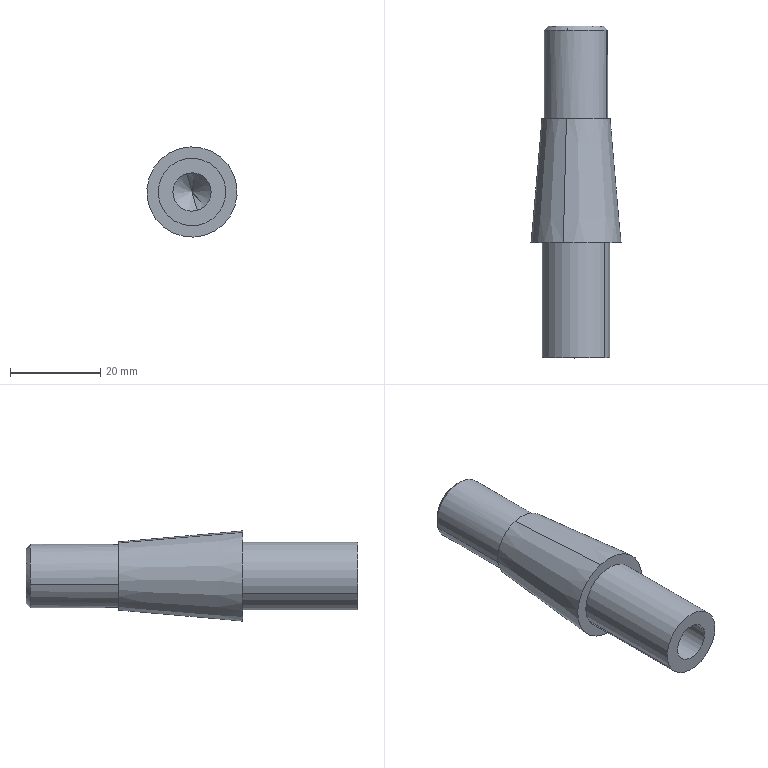Part | SolidWorks | features BaseBody 1 | 1 solid | 16 faces | box 20 x 73.5 x 20 mm | volume 13373 mm3 | cone 6 | cylinder 6 | plane 4 | commonest cylinder face diameters 8.5 x2 14 x2 14.95 x2
STEP:
#1=CARTESIAN_POINT('',(-385.826,-48.,37.663));
#2=VERTEX_POINT('',#1);
#3=CARTESIAN_POINT('',(-389.222,-48.,49.277));
#4=VERTEX_POINT('',#3);
#5=CARTESIAN_POINT('',(-387.524,-48.,43.47));
#6=DIRECTION('',(0.,1.,0.));
#7=DIRECTION('',(-0.9598,0.,-0.2807));
#8=AXIS2_PLACEMENT_3D('',#5,#6,#7);
#9=CIRCLE('',#8,6.05);
#10=EDGE_CURVE('',#2,#4,#9,.T.);
#11=ORIENTED_EDGE('',*,*,#10,.F.);
#12=CARTESIAN_POINT('',(-385.56,-48.95,36.751));
#13=VERTEX_POINT('',#12);
#14=CARTESIAN_POINT('',(-385.693,-48.475,37.207));
#15=DIRECTION('',(0.1985,-0.7071,-0.6787));
#16=VECTOR('',#15,1000.);
#17=LINE('',#14,#16);
#18=EDGE_CURVE('',#2,#13,#17,.T.);
#19=ORIENTED_EDGE('',*,*,#18,.T.);
#20=CARTESIAN_POINT('',(-394.243,-48.95,41.505));
#21=VERTEX_POINT('',#20);
#22=CARTESIAN_POINT('',(-387.524,-48.95,43.47));
#23=DIRECTION('',(0.,1.,0.));
#24=DIRECTION('',(-0.9598,0.,-0.2807));
#25=AXIS2_PLACEMENT_3D('',#22,#23,#24);
#26=CIRCLE('',#25,7.);
#27=EDGE_CURVE('',#13,#21,#26,.T.);
#28=ORIENTED_EDGE('',*,*,#27,.T.);
#29=CARTESIAN_POINT('',(-389.489,-48.95,50.189));
#30=VERTEX_POINT('',#29);
#31=CARTESIAN_POINT('',(-387.524,-48.95,43.47));
#32=DIRECTION('',(0.,1.,0.));
#33=DIRECTION('',(-0.9598,0.,-0.2807));
#34=AXIS2_PLACEMENT_3D('',#31,#32,#33);
#35=CIRCLE('',#34,7.);
#36=EDGE_CURVE('',#21,#30,#35,.T.);
#37=ORIENTED_EDGE('',*,*,#36,.T.);
#38=CARTESIAN_POINT('',(-389.356,-48.475,49.733));
#39=DIRECTION('',(-0.1985,-0.7071,0.6787));
#40=VECTOR('',#39,1000.);
#41=LINE('',#38,#40);
#42=EDGE_CURVE('',#4,#30,#41,.T.);
#43=ORIENTED_EDGE('',*,*,#42,.F.);
#44=EDGE_LOOP('',(#11,#19,#28,#37,#43));
#45=FACE_OUTER_BOUND('',#44,.T.);
#46=CARTESIAN_POINT('',(-387.524,-48.475,43.47));
#47=DIRECTION('',(0.,-1.,0.));
#48=DIRECTION('',(-0.2807,0.,0.9598));
#49=AXIS2_PLACEMENT_3D('',#46,#47,#48);
#50=CONICAL_SURFACE('',#49,6.525,0.7854);
#51=ADVANCED_FACE('',(#45),#50,.T.);
#52=CARTESIAN_POINT('',(-387.524,-102.,43.47));
#53=VERTEX_POINT('',#52);
#54=CARTESIAN_POINT('',(-388.717,-106.25,47.549));
#55=VERTEX_POINT('',#54);
#56=CARTESIAN_POINT('',(-388.133,-104.168,45.55));
#57=DIRECTION('',(-0.1985,-0.7071,0.6787));
#58=VECTOR('',#57,1000.);
#59=LINE('',#56,#58);
#60=EDGE_CURVE('',#53,#55,#59,.T.);
#61=ORIENTED_EDGE('',*,*,#60,.F.);
#62=CARTESIAN_POINT('',(-386.332,-106.25,39.391));
#63=VERTEX_POINT('',#62);
#64=CARTESIAN_POINT('',(-386.916,-104.168,41.39));
#65=DIRECTION('',(0.1985,-0.7071,-0.6787));
#66=VECTOR('',#65,1000.);
#67=LINE('',#64,#66);
#68=EDGE_CURVE('',#53,#63,#67,.T.);
#69=ORIENTED_EDGE('',*,*,#68,.T.);
#70=CARTESIAN_POINT('',(-383.445,-106.25,44.663));
#71=VERTEX_POINT('',#70);
#72=CARTESIAN_POINT('',(-387.524,-106.25,43.47));
#73=DIRECTION('',(0.,1.,0.));
#74=DIRECTION('',(-0.9598,0.,-0.2807));
#75=AXIS2_PLACEMENT_3D('',#72,#73,#74);
#76=CIRCLE('',#75,4.25);
#77=EDGE_CURVE('',#71,#63,#76,.T.);
#78=ORIENTED_EDGE('',*,*,#77,.F.);
#79=CARTESIAN_POINT('',(-387.524,-106.25,43.47));
#80=DIRECTION('',(0.,1.,0.));
#81=DIRECTION('',(-0.9598,0.,-0.2807));
#82=AXIS2_PLACEMENT_3D('',#79,#80,#81);
#83=CIRCLE('',#82,4.25);
#84=EDGE_CURVE('',#55,#71,#83,.T.);
#85=ORIENTED_EDGE('',*,*,#84,.F.);
#86=EDGE_LOOP('',(#61,#69,#78,#85));
#87=FACE_OUTER_BOUND('',#86,.T.);
#88=CARTESIAN_POINT('',(-387.524,-104.168,43.47));
#89=DIRECTION('',(0.,-1.,0.));
#90=DIRECTION('',(-0.2807,0.,0.9598));
#91=AXIS2_PLACEMENT_3D('',#88,#89,#90);
#92=CONICAL_SURFACE('',#91,2.168,0.7854);
#93=ADVANCED_FACE('',(#87),#92,.F.);
#94=CARTESIAN_POINT('',(-391.604,-106.25,42.277));
#95=VERTEX_POINT('',#94);
#96=CARTESIAN_POINT('',(-387.524,-106.25,43.47));
#97=DIRECTION('',(0.,1.,0.));
#98=DIRECTION('',(-0.9598,0.,-0.2807));
#99=AXIS2_PLACEMENT_3D('',#96,#97,#98);
#100=CIRCLE('',#99,4.25);
#101=EDGE_CURVE('',#95,#55,#100,.T.);
#102=ORIENTED_EDGE('',*,*,#101,.T.);
#103=ORIENTED_EDGE('',*,*,#84,.T.);
#104=CARTESIAN_POINT('',(-383.445,-121.5,44.663));
#105=VERTEX_POINT('',#104);
#106=CARTESIAN_POINT('',(-383.445,-122.,44.663));
#107=DIRECTION('',(0.,-1.,0.));
#108=VECTOR('',#107,1000.);
#109=LINE('',#106,#108);
#110=EDGE_CURVE('',#71,#105,#109,.T.);
#111=ORIENTED_EDGE('',*,*,#110,.T.);
#112=CARTESIAN_POINT('',(-391.604,-121.5,42.277));
#113=VERTEX_POINT('',#112);
#114=CARTESIAN_POINT('',(-387.524,-121.5,43.47));
#115=DIRECTION('',(0.,1.,0.));
#116=DIRECTION('',(-0.9598,0.,-0.2807));
#117=AXIS2_PLACEMENT_3D('',#114,#115,#116);
#118=CIRCLE('',#117,4.25);
#119=EDGE_CURVE('',#113,#105,#118,.T.);
#120=ORIENTED_EDGE('',*,*,#119,.F.);
#121=CARTESIAN_POINT('',(-391.604,-122.,42.277));
#122=DIRECTION('',(0.,-1.,0.));
#123=VECTOR('',#122,1000.);
#124=LINE('',#121,#123);
#125=EDGE_CURVE('',#95,#113,#124,.T.);
#126=ORIENTED_EDGE('',*,*,#125,.F.);
#127=EDGE_LOOP('',(#102,#103,#111,#120,#126));
#128=FACE_OUTER_BOUND('',#127,.T.);
#129=CARTESIAN_POINT('',(-387.524,-122.,43.47));
#130=DIRECTION('',(0.,-1.,0.));
#131=DIRECTION('',(-0.9598,0.,-0.2807));
#132=AXIS2_PLACEMENT_3D('',#129,#130,#131);
#133=CYLINDRICAL_SURFACE('',#132,4.25);
#134=ADVANCED_FACE('',(#128),#133,.F.);
#135=CARTESIAN_POINT('',(-381.159,-96.,47.389));
#136=VERTEX_POINT('',#135);
#137=CARTESIAN_POINT('',(-393.89,-96.,39.551));
#138=VERTEX_POINT('',#137);
#139=CARTESIAN_POINT('',(-387.524,-96.,43.47));
#140=DIRECTION('',(0.,1.,0.));
#141=DIRECTION('',(0.8515,0.,0.5243));
#142=AXIS2_PLACEMENT_3D('',#139,#140,#141);
#143=CIRCLE('',#142,7.475);
#144=EDGE_CURVE('',#136,#138,#143,.T.);
#145=ORIENTED_EDGE('',*,*,#144,.F.);
#146=CARTESIAN_POINT('',(-381.159,-121.5,47.389));
#147=VERTEX_POINT('',#146);
#148=CARTESIAN_POINT('',(-381.159,-122.,47.389));
#149=DIRECTION('',(0.,-1.,0.));
#150=VECTOR('',#149,1000.);
#151=LINE('',#148,#150);
#152=EDGE_CURVE('',#136,#147,#151,.T.);
#153=ORIENTED_EDGE('',*,*,#152,.T.);
#154=CARTESIAN_POINT('',(-393.89,-121.5,39.551));
#155=VERTEX_POINT('',#154);
#156=CARTESIAN_POINT('',(-387.524,-121.5,43.47));
#157=DIRECTION('',(0.,-1.,0.));
#158=DIRECTION('',(0.,0.,-1.));
#159=AXIS2_PLACEMENT_3D('',#156,#157,#158);
#160=CIRCLE('',#159,7.475);
#161=EDGE_CURVE('',#155,#147,#160,.T.);
#162=ORIENTED_EDGE('',*,*,#161,.F.);
#163=CARTESIAN_POINT('',(-393.89,-122.,39.551));
#164=DIRECTION('',(0.,-1.,0.));
#165=VECTOR('',#164,1000.);
#166=LINE('',#163,#165);
#167=EDGE_CURVE('',#138,#155,#166,.T.);
#168=ORIENTED_EDGE('',*,*,#167,.F.);
#169=EDGE_LOOP('',(#145,#153,#162,#168));
#170=FACE_OUTER_BOUND('',#169,.T.);
#171=CARTESIAN_POINT('',(-387.524,-122.,43.47));
#172=DIRECTION('',(0.,-1.,0.));
#173=DIRECTION('',(-0.8515,0.,-0.5243));
#174=AXIS2_PLACEMENT_3D('',#171,#172,#173);
#175=CYLINDRICAL_SURFACE('',#174,7.475);
#176=ADVANCED_FACE('',(#170),#175,.T.);
#177=CARTESIAN_POINT('',(-394.243,-68.5,41.505));
#178=VERTEX_POINT('',#177);
#179=CARTESIAN_POINT('',(-380.806,-68.5,45.435));
#180=VERTEX_POINT('',#179);
#181=CARTESIAN_POINT('',(-387.524,-68.5,43.47));
#182=DIRECTION('',(0.,-1.,0.));
#183=DIRECTION('',(0.9598,0.,0.2807));
#184=AXIS2_PLACEMENT_3D('',#181,#182,#183);
#185=CIRCLE('',#184,7.);
#186=EDGE_CURVE('',#178,#180,#185,.T.);
#187=ORIENTED_EDGE('',*,*,#186,.F.);
#188=CARTESIAN_POINT('',(-394.243,-63.,41.505));
#189=DIRECTION('',(0.,1.,0.));
#190=VECTOR('',#189,1000.);
#191=LINE('',#188,#190);
#192=EDGE_CURVE('',#178,#21,#191,.T.);
#193=ORIENTED_EDGE('',*,*,#192,.T.);
#194=ORIENTED_EDGE('',*,*,#27,.F.);
#195=CARTESIAN_POINT('',(-380.806,-48.95,45.435));
#196=VERTEX_POINT('',#195);
#197=CARTESIAN_POINT('',(-387.524,-48.95,43.47));
#198=DIRECTION('',(0.,1.,0.));
#199=DIRECTION('',(-0.9598,0.,-0.2807));
#200=AXIS2_PLACEMENT_3D('',#197,#198,#199);
#201=CIRCLE('',#200,7.);
#202=EDGE_CURVE('',#196,#13,#201,.T.);
#203=ORIENTED_EDGE('',*,*,#202,.F.);
#204=CARTESIAN_POINT('',(-380.806,-63.,45.435));
#205=DIRECTION('',(0.,1.,0.));
#206=VECTOR('',#205,1000.);
#207=LINE('',#204,#206);
#208=EDGE_CURVE('',#180,#196,#207,.T.);
#209=ORIENTED_EDGE('',*,*,#208,.F.);
#210=EDGE_LOOP('',(#187,#193,#194,#203,#209));
#211=FACE_OUTER_BOUND('',#210,.T.);
#212=CARTESIAN_POINT('',(-387.524,-63.,43.47));
#213=DIRECTION('',(0.,1.,0.));
#214=DIRECTION('',(0.9598,0.,0.2807));
#215=AXIS2_PLACEMENT_3D('',#212,#213,#214);
#216=CYLINDRICAL_SURFACE('',#215,7.);
#217=ADVANCED_FACE('',(#211),#216,.T.);
#218=CARTESIAN_POINT('',(-389.647,-68.5,50.73));
#219=VERTEX_POINT('',#218);
#220=CARTESIAN_POINT('',(-385.402,-68.5,36.21));
#221=VERTEX_POINT('',#220);
#222=CARTESIAN_POINT('',(-387.524,-68.5,43.47));
#223=DIRECTION('',(0.,-1.,0.));
#224=DIRECTION('',(-0.2807,0.,0.9598));
#225=AXIS2_PLACEMENT_3D('',#222,#223,#224);
#226=CIRCLE('',#225,7.564);
#227=EDGE_CURVE('',#219,#221,#226,.T.);
#228=ORIENTED_EDGE('',*,*,#227,.T.);
#229=CARTESIAN_POINT('',(-384.718,-96.,33.872));
#230=VERTEX_POINT('',#229);
#231=CARTESIAN_POINT('',(-385.06,-82.25,35.041));
#232=DIRECTION('',(0.02477,-0.9961,-0.0847));
#233=VECTOR('',#232,1000.);
#234=LINE('',#231,#233);
#235=EDGE_CURVE('',#221,#230,#234,.T.);
#236=ORIENTED_EDGE('',*,*,#235,.T.);
#237=CARTESIAN_POINT('',(-390.331,-96.,53.068));
#238=VERTEX_POINT('',#237);
#239=CARTESIAN_POINT('',(-387.524,-96.,43.47));
#240=DIRECTION('',(0.,-1.,0.));
#241=DIRECTION('',(0.2807,0.,-0.9598));
#242=AXIS2_PLACEMENT_3D('',#239,#240,#241);
#243=CIRCLE('',#242,10.);
#244=EDGE_CURVE('',#238,#230,#243,.T.);
#245=ORIENTED_EDGE('',*,*,#244,.F.);
#246=CARTESIAN_POINT('',(-389.989,-82.25,51.899));
#247=DIRECTION('',(-0.02477,-0.9961,0.0847));
#248=VECTOR('',#247,1000.);
#249=LINE('',#246,#248);
#250=EDGE_CURVE('',#219,#238,#249,.T.);
#251=ORIENTED_EDGE('',*,*,#250,.F.);
#252=EDGE_LOOP('',(#228,#236,#245,#251));
#253=FACE_OUTER_BOUND('',#252,.T.);
#254=CARTESIAN_POINT('',(-387.524,-82.25,43.47));
#255=DIRECTION('',(0.,-1.,0.));
#256=DIRECTION('',(-0.2807,0.,0.9598));
#257=AXIS2_PLACEMENT_3D('',#254,#255,#256);
#258=CONICAL_SURFACE('',#257,8.782,0.08837);
#259=ADVANCED_FACE('',(#253),#258,.T.);
#260=ORIENTED_EDGE('',*,*,#119,.T.);
#261=CARTESIAN_POINT('',(-387.524,-121.5,43.47));
#262=DIRECTION('',(0.,1.,0.));
#263=DIRECTION('',(-0.9598,0.,-0.2807));
#264=AXIS2_PLACEMENT_3D('',#261,#262,#263);
#265=CIRCLE('',#264,4.25);
#266=EDGE_CURVE('',#105,#113,#265,.T.);
#267=ORIENTED_EDGE('',*,*,#266,.T.);
#268=EDGE_LOOP('',(#260,#267));
#269=FACE_BOUND('',#268,.T.);
#270=ORIENTED_EDGE('',*,*,#161,.T.);
#271=CARTESIAN_POINT('',(-387.524,-121.5,43.47));
#272=DIRECTION('',(0.,-1.,0.));
#273=DIRECTION('',(0.,0.,-1.));
#274=AXIS2_PLACEMENT_3D('',#271,#272,#273);
#275=CIRCLE('',#274,7.475);
#276=EDGE_CURVE('',#147,#155,#275,.T.);
#277=ORIENTED_EDGE('',*,*,#276,.T.);
#278=EDGE_LOOP('',(#270,#277));
#279=FACE_OUTER_BOUND('',#278,.T.);
#280=CARTESIAN_POINT('',(-449.261,-121.5,5.459));
#281=DIRECTION('',(0.,-1.,0.));
#282=DIRECTION('',(0.,0.,-1.));
#283=AXIS2_PLACEMENT_3D('',#280,#281,#282);
#284=PLANE('',#283);
#285=ADVANCED_FACE('',(#269,#279),#284,.T.);
#286=CARTESIAN_POINT('',(-387.524,-96.,43.47));
#287=DIRECTION('',(0.,1.,0.));
#288=DIRECTION('',(0.8515,0.,0.5243));
#289=AXIS2_PLACEMENT_3D('',#286,#287,#288);
#290=CIRCLE('',#289,7.475);
#291=EDGE_CURVE('',#138,#136,#290,.T.);
#292=ORIENTED_EDGE('',*,*,#291,.T.);
#293=ORIENTED_EDGE('',*,*,#144,.T.);
#294=EDGE_LOOP('',(#292,#293));
#295=FACE_BOUND('',#294,.T.);
#296=ORIENTED_EDGE('',*,*,#244,.T.);
#297=CARTESIAN_POINT('',(-387.524,-96.,43.47));
#298=DIRECTION('',(0.,-1.,0.));
#299=DIRECTION('',(0.2807,0.,-0.9598));
#300=AXIS2_PLACEMENT_3D('',#297,#298,#299);
#301=CIRCLE('',#300,10.);
#302=EDGE_CURVE('',#230,#238,#301,.T.);
#303=ORIENTED_EDGE('',*,*,#302,.T.);
#304=EDGE_LOOP('',(#296,#303));
#305=FACE_OUTER_BOUND('',#304,.T.);
#306=CARTESIAN_POINT('',(-387.524,-96.,43.47));
#307=DIRECTION('',(0.,-1.,0.));
#308=DIRECTION('',(0.,0.,-1.));
#309=AXIS2_PLACEMENT_3D('',#306,#307,#308);
#310=PLANE('',#309);
#311=ADVANCED_FACE('',(#295,#305),#310,.T.);
#312=ORIENTED_EDGE('',*,*,#235,.F.);
#313=CARTESIAN_POINT('',(-387.524,-68.5,43.47));
#314=DIRECTION('',(0.,-1.,0.));
#315=DIRECTION('',(-0.2807,0.,0.9598));
#316=AXIS2_PLACEMENT_3D('',#313,#314,#315);
#317=CIRCLE('',#316,7.564);
#318=EDGE_CURVE('',#221,#219,#317,.T.);
#319=ORIENTED_EDGE('',*,*,#318,.T.);
#320=ORIENTED_EDGE('',*,*,#250,.T.);
#321=ORIENTED_EDGE('',*,*,#302,.F.);
#322=EDGE_LOOP('',(#312,#319,#320,#321));
#323=FACE_OUTER_BOUND('',#322,.T.);
#324=CARTESIAN_POINT('',(-387.524,-82.25,43.47));
#325=DIRECTION('',(0.,-1.,0.));
#326=DIRECTION('',(-0.2807,0.,0.9598));
#327=AXIS2_PLACEMENT_3D('',#324,#325,#326);
#328=CONICAL_SURFACE('',#327,8.782,0.08837);
#329=ADVANCED_FACE('',(#323),#328,.T.);
#330=CARTESIAN_POINT('',(-387.524,-68.5,43.47));
#331=DIRECTION('',(0.,-1.,0.));
#332=DIRECTION('',(0.9598,0.,0.2807));
#333=AXIS2_PLACEMENT_3D('',#330,#331,#332);
#334=CIRCLE('',#333,7.);
#335=EDGE_CURVE('',#180,#178,#334,.T.);
#336=ORIENTED_EDGE('',*,*,#335,.T.);
#337=ORIENTED_EDGE('',*,*,#186,.T.);
#338=EDGE_LOOP('',(#336,#337));
#339=FACE_BOUND('',#338,.T.);
#340=ORIENTED_EDGE('',*,*,#227,.F.);
#341=ORIENTED_EDGE('',*,*,#318,.F.);
#342=EDGE_LOOP('',(#340,#341));
#343=FACE_OUTER_BOUND('',#342,.T.);
#344=CARTESIAN_POINT('',(5.879,-68.5,101.935));
#345=DIRECTION('',(0.,1.,0.));
#346=DIRECTION('',(1.,0.,0.));
#347=AXIS2_PLACEMENT_3D('',#344,#345,#346);
#348=PLANE('',#347);
#349=ADVANCED_FACE('',(#339,#343),#348,.T.);
#350=ORIENTED_EDGE('',*,*,#192,.F.);
#351=ORIENTED_EDGE('',*,*,#335,.F.);
#352=ORIENTED_EDGE('',*,*,#208,.T.);
#353=CARTESIAN_POINT('',(-387.524,-48.95,43.47));
#354=DIRECTION('',(0.,1.,0.));
#355=DIRECTION('',(-0.9598,0.,-0.2807));
#356=AXIS2_PLACEMENT_3D('',#353,#354,#355);
#357=CIRCLE('',#356,7.);
#358=EDGE_CURVE('',#30,#196,#357,.T.);
#359=ORIENTED_EDGE('',*,*,#358,.F.);
#360=ORIENTED_EDGE('',*,*,#36,.F.);
#361=EDGE_LOOP('',(#350,#351,#352,#359,#360));
#362=FACE_OUTER_BOUND('',#361,.T.);
#363=CARTESIAN_POINT('',(-387.524,-63.,43.47));
#364=DIRECTION('',(0.,1.,0.));
#365=DIRECTION('',(0.9598,0.,0.2807));
#366=AXIS2_PLACEMENT_3D('',#363,#364,#365);
#367=CYLINDRICAL_SURFACE('',#366,7.);
#368=ADVANCED_FACE('',(#362),#367,.T.);
#369=CARTESIAN_POINT('',(-387.524,-48.,43.47));
#370=DIRECTION('',(0.,1.,0.));
#371=DIRECTION('',(-0.9598,0.,-0.2807));
#372=AXIS2_PLACEMENT_3D('',#369,#370,#371);
#373=CIRCLE('',#372,6.05);
#374=EDGE_CURVE('',#4,#2,#373,.T.);
#375=ORIENTED_EDGE('',*,*,#374,.T.);
#376=ORIENTED_EDGE('',*,*,#10,.T.);
#377=EDGE_LOOP('',(#375,#376));
#378=FACE_OUTER_BOUND('',#377,.T.);
#379=CARTESIAN_POINT('',(5.879,-48.,101.935));
#380=DIRECTION('',(0.,1.,0.));
#381=DIRECTION('',(1.,0.,0.));
#382=AXIS2_PLACEMENT_3D('',#379,#380,#381);
#383=PLANE('',#382);
#384=ADVANCED_FACE('',(#378),#383,.T.);
#385=ORIENTED_EDGE('',*,*,#152,.F.);
#386=ORIENTED_EDGE('',*,*,#291,.F.);
#387=ORIENTED_EDGE('',*,*,#167,.T.);
#388=ORIENTED_EDGE('',*,*,#276,.F.);
#389=EDGE_LOOP('',(#385,#386,#387,#388));
#390=FACE_OUTER_BOUND('',#389,.T.);
#391=CARTESIAN_POINT('',(-387.524,-122.,43.47));
#392=DIRECTION('',(0.,-1.,0.));
#393=DIRECTION('',(-0.8515,0.,-0.5243));
#394=AXIS2_PLACEMENT_3D('',#391,#392,#393);
#395=CYLINDRICAL_SURFACE('',#394,7.475);
#396=ADVANCED_FACE('',(#390),#395,.T.);
#397=ORIENTED_EDGE('',*,*,#110,.F.);
#398=ORIENTED_EDGE('',*,*,#77,.T.);
#399=CARTESIAN_POINT('',(-387.524,-106.25,43.47));
#400=DIRECTION('',(0.,1.,0.));
#401=DIRECTION('',(-0.9598,0.,-0.2807));
#402=AXIS2_PLACEMENT_3D('',#399,#400,#401);
#403=CIRCLE('',#402,4.25);
#404=EDGE_CURVE('',#63,#95,#403,.T.);
#405=ORIENTED_EDGE('',*,*,#404,.T.);
#406=ORIENTED_EDGE('',*,*,#125,.T.);
#407=ORIENTED_EDGE('',*,*,#266,.F.);
#408=EDGE_LOOP('',(#397,#398,#405,#406,#407));
#409=FACE_OUTER_BOUND('',#408,.T.);
#410=CARTESIAN_POINT('',(-387.524,-122.,43.47));
#411=DIRECTION('',(0.,-1.,0.));
#412=DIRECTION('',(-0.9598,0.,-0.2807));
#413=AXIS2_PLACEMENT_3D('',#410,#411,#412);
#414=CYLINDRICAL_SURFACE('',#413,4.25);
#415=ADVANCED_FACE('',(#409),#414,.F.);
#416=ORIENTED_EDGE('',*,*,#68,.F.);
#417=ORIENTED_EDGE('',*,*,#60,.T.);
#418=ORIENTED_EDGE('',*,*,#101,.F.);
#419=ORIENTED_EDGE('',*,*,#404,.F.);
#420=EDGE_LOOP('',(#416,#417,#418,#419));
#421=FACE_OUTER_BOUND('',#420,.T.);
#422=CARTESIAN_POINT('',(-387.524,-104.168,43.47));
#423=DIRECTION('',(0.,-1.,0.));
#424=DIRECTION('',(-0.2807,0.,0.9598));
#425=AXIS2_PLACEMENT_3D('',#422,#423,#424);
#426=CONICAL_SURFACE('',#425,2.168,0.7854);
#427=ADVANCED_FACE('',(#421),#426,.F.);
#428=ORIENTED_EDGE('',*,*,#18,.F.);
#429=ORIENTED_EDGE('',*,*,#374,.F.);
#430=ORIENTED_EDGE('',*,*,#42,.T.);
#431=ORIENTED_EDGE('',*,*,#358,.T.);
#432=ORIENTED_EDGE('',*,*,#202,.T.);
#433=EDGE_LOOP('',(#428,#429,#430,#431,#432));
#434=FACE_OUTER_BOUND('',#433,.T.);
#435=CARTESIAN_POINT('',(-387.524,-48.475,43.47));
#436=DIRECTION('',(0.,-1.,0.));
#437=DIRECTION('',(-0.2807,0.,0.9598));
#438=AXIS2_PLACEMENT_3D('',#435,#436,#437);
#439=CONICAL_SURFACE('',#438,6.525,0.7854);
#440=ADVANCED_FACE('',(#434),#439,.T.);
#441=CLOSED_SHELL('',(#51,#93,#134,#176,#217,#259,#285,#311,#329,#349,#368,#384,#396,#415,#427,#440));
#442=MANIFOLD_SOLID_BREP('',#441);
#443=CARTESIAN_POINT('',(0.,0.,0.));
#444=DIRECTION('',(0.,0.,1.));
#445=DIRECTION('',(1.,0.,0.));
#446=AXIS2_PLACEMENT_3D('',#443,#444,#445);
#447=(LENGTH_UNIT()NAMED_UNIT(*)SI_UNIT(.MILLI.,.METRE.));
#448=UNCERTAINTY_MEASURE_WITH_UNIT(LENGTH_MEASURE(0.00001),#447,'','');
#449=(NAMED_UNIT(*)PLANE_ANGLE_UNIT()SI_UNIT($,.RADIAN.));
#450=(NAMED_UNIT(*)SI_UNIT($,.STERADIAN.)SOLID_ANGLE_UNIT());
#451=(GEOMETRIC_REPRESENTATION_CONTEXT(3)GLOBAL_UNCERTAINTY_ASSIGNED_CONTEXT((#448))GLOBAL_UNIT_ASSIGNED_CONTEXT((#447,#449,#450))REPRESENTATION_CONTEXT('',''));
#452=ADVANCED_BREP_SHAPE_REPRESENTATION('',(#442,#446),#451);